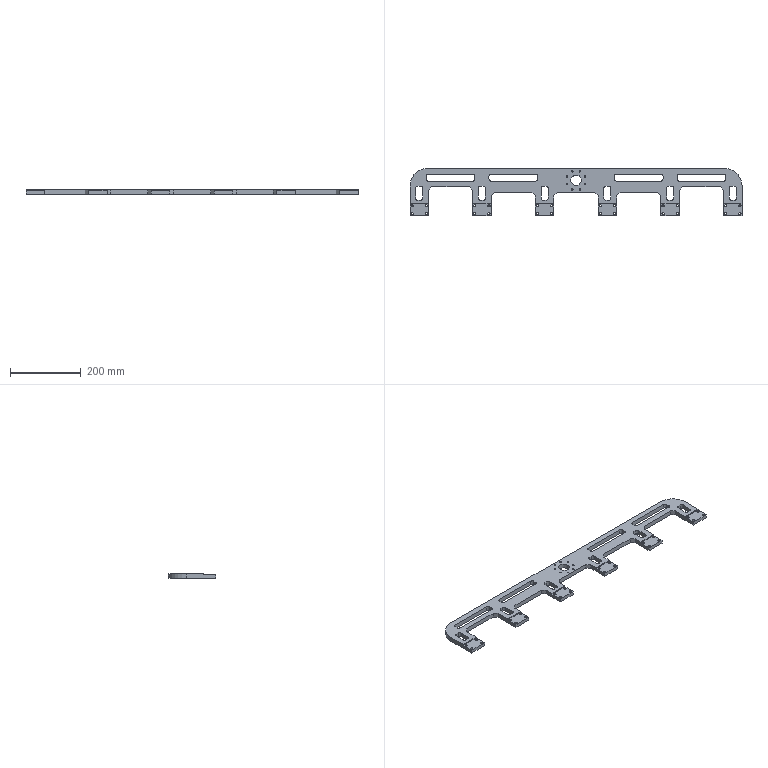NC program | NX | posted with a generic post | part box 941 x 134 x 13 mm
Lines 100 to 1108 of 8798:
(ZLEVEL_PROFILE_COPY_3 , TOOL : D10)
N180 T10 M6
N182 G54
N184 G17 G0 G90 X65.687 Y-75.6 S9500 M3
N186 G43 Z30. H10
N188 Z4.036
N190 G94 G1 Z-0.964 F1000.
N192 X63.955 Y-72.6
N194 G3 X63.089 Y-72.1 R1.
N196 G1 X62.9 F3500.
N198 G2 X57.8 Y-67. R5.1
N200 G1 Y-13.067
N202 X50.788 Y-6.055
N204 X-50.788
N206 X-57.8 Y-13.067
N208 Y-67.
N210 G2 X-62.9 Y-72.1 R5.1
N212 G1 X-114.9
N214 G2 X-120. Y-67. R5.1
N216 G1 Y-13.067
N218 X-127.012 Y-6.055
N220 X-228.588
N222 X-235.6 Y-13.067
N224 Y-67.
N226 G2 X-240.7 Y-72.1 R5.1
N228 G1 X-292.7
N230 G2 X-297.8 Y-67. R5.1
N232 G1 Y2.888
N234 X-304.812 Y9.9
N236 X-406.388
N238 X-413.4 Y2.888
N240 Y-67.
N242 G2 X-418.5 Y-72.1 R5.1
N244 G1 X-470.5
N246 G2 X-475.6 Y-67. R5.1
N248 G1 Y17.
N250 G2 X-420.5 Y72.1 R55.1
N252 G1 X63.089
N254 G3 X63.955 Y72.6 R1.
N256 G1 X65.687 Y75.6
N258 Z4.036
N260 G0 Z30.
N262 Z3.071
N264 G1 Z-1.929 F1000.
N266 X63.955 Y72.6
N268 G2 X63.089 Y72.1 R1.
N270 G1 X-420.5 F3500.
N272 G3 X-475.6 Y17. R55.1
N274 G1 Y-67.
N276 G3 X-470.5 Y-72.1 R5.1
N278 G1 X-418.5
N280 G3 X-413.4 Y-67. R5.1
N282 G1 Y2.888
N284 X-406.388 Y9.9
N286 X-304.812
N288 X-297.8 Y2.888
N290 Y-67.
N292 G3 X-292.7 Y-72.1 R5.1
N294 G1 X-240.7
N296 G3 X-235.6 Y-67. R5.1
N298 G1 Y-13.067
N300 X-228.588 Y-6.055
N302 X-127.012
N304 X-120. Y-13.067
N306 Y-67.
N308 G3 X-114.9 Y-72.1 R5.1
N310 G1 X-62.9
N312 G3 X-57.8 Y-67. R5.1
N314 G1 Y-13.067
N316 X-50.788 Y-6.055
N318 X50.788
N320 X57.8 Y-13.067
N322 Y-67.
N324 G3 X62.9 Y-72.1 R5.1
N326 G1 X63.089
N328 G2 X63.955 Y-72.6 R1.
N330 G1 X65.687 Y-75.6
N332 Z3.071
N334 G0 Z30.
N336 Z2.107
N338 G1 Z-2.893 F1000.
N340 X63.955 Y-72.6
N342 G3 X63.089 Y-72.1 R1.
N344 G1 X62.9 F3500.
N346 G2 X57.8 Y-67. R5.1
N348 G1 Y-13.067
N350 X50.788 Y-6.055
N352 X-50.788
N354 X-57.8 Y-13.067
N356 Y-67.
N358 G2 X-62.9 Y-72.1 R5.1
N360 G1 X-114.9
N362 G2 X-120. Y-67. R5.1
N364 G1 Y-13.067
N366 X-127.012 Y-6.055
N368 X-228.588
N370 X-235.6 Y-13.067
N372 Y-67.
N374 G2 X-240.7 Y-72.1 R5.1
N376 G1 X-292.7
N378 G2 X-297.8 Y-67. R5.1
N380 G1 Y2.888
N382 X-304.812 Y9.9
N384 X-406.388
N386 X-413.4 Y2.888
N388 Y-67.
N390 G2 X-418.5 Y-72.1 R5.1
N392 G1 X-470.5
N394 G2 X-475.6 Y-67. R5.1
N396 G1 Y17.
N398 G2 X-420.5 Y72.1 R55.1
N400 G1 X63.089
N402 G3 X63.955 Y72.6 R1.
N404 G1 X65.687 Y75.6
N406 Z2.107
N408 G0 Z30.
N410 Z1.143
N412 G1 Z-3.857 F1000.
N414 X63.955 Y72.6
N416 G2 X63.089 Y72.1 R1.
N418 G1 X-420.5 F3500.
N420 G3 X-475.6 Y17. R55.1
N422 G1 Y-67.
N424 G3 X-470.5 Y-72.1 R5.1
N426 G1 X-418.5
N428 G3 X-413.4 Y-67. R5.1
N430 G1 Y2.888
N432 X-406.388 Y9.9
N434 X-304.812
N436 X-297.8 Y2.888
N438 Y-67.
N440 G3 X-292.7 Y-72.1 R5.1
N442 G1 X-240.7
N444 G3 X-235.6 Y-67. R5.1
N446 G1 Y-13.067
N448 X-228.588 Y-6.055
N450 X-127.012
N452 X-120. Y-13.067
N454 Y-67.
N456 G3 X-114.9 Y-72.1 R5.1
N458 G1 X-62.9
N460 G3 X-57.8 Y-67. R5.1
N462 G1 Y-13.067
N464 X-50.788 Y-6.055
N466 X50.788
N468 X57.8 Y-13.067
N470 Y-67.
N472 G3 X62.9 Y-72.1 R5.1
N474 G1 X63.089
N476 G2 X63.955 Y-72.6 R1.
N478 G1 X65.687 Y-75.6
N480 Z1.143
N482 G0 Z30.
N484 Z0.179
N486 G1 Z-4.821 F1000.
N488 X63.955 Y-72.6
N490 G3 X63.089 Y-72.1 R1.
N492 G1 X62.9 F3500.
N494 G2 X57.8 Y-67. R5.1
N496 G1 Y-13.067
N498 X50.788 Y-6.055
N500 X-50.788
N502 X-57.8 Y-13.067
N504 Y-67.
N506 G2 X-62.9 Y-72.1 R5.1
N508 G1 X-114.9
N510 G2 X-120. Y-67. R5.1
N512 G1 Y-13.067
N514 X-127.012 Y-6.055
N516 X-228.588
N518 X-235.6 Y-13.067
N520 Y-67.
N522 G2 X-240.7 Y-72.1 R5.1
N524 G1 X-292.7
N526 G2 X-297.8 Y-67. R5.1
N528 G1 Y2.888
N530 X-304.812 Y9.9
N532 X-406.388
N534 X-413.4 Y2.888
N536 Y-67.
N538 G2 X-418.5 Y-72.1 R5.1
N540 G1 X-470.5
N542 G2 X-475.6 Y-67. R5.1
N544 G1 Y17.
N546 G2 X-420.5 Y72.1 R55.1
N548 G1 X63.089
N550 G3 X63.955 Y72.6 R1.
N552 G1 X65.687 Y75.6
N554 Z0.179
N556 G0 Z30.
N558 Z-0.786
N560 G1 Z-5.786 F1000.
N562 X63.955 Y72.6
N564 G2 X63.089 Y72.1 R1.
N566 G1 X-420.5 F3500.
N568 G3 X-475.6 Y17. R55.1
N570 G1 Y-67.
N572 G3 X-470.5 Y-72.1 R5.1
N574 G1 X-418.5
N576 G3 X-413.4 Y-67. R5.1
N578 G1 Y2.888
N580 X-406.388 Y9.9
N582 X-304.812
N584 X-297.8 Y2.888
N586 Y-67.
N588 G3 X-292.7 Y-72.1 R5.1
N590 G1 X-240.7
N592 G3 X-235.6 Y-67. R5.1
N594 G1 Y-13.067
N596 X-228.588 Y-6.055
N598 X-127.012
N600 X-120. Y-13.067
N602 Y-67.
N604 G3 X-114.9 Y-72.1 R5.1
N606 G1 X-62.9
N608 G3 X-57.8 Y-67. R5.1
N610 G1 Y-13.067
N612 X-50.788 Y-6.055
N614 X50.788
N616 X57.8 Y-13.067
N618 Y-67.
N620 G3 X62.9 Y-72.1 R5.1
N622 G1 X63.089
N624 G2 X63.955 Y-72.6 R1.
N626 G1 X65.687 Y-75.6
N628 Z-0.786
N630 G0 Z30.
N632 Z-1.75
N634 G1 Z-6.75 F1000.
N636 X63.955 Y-72.6
N638 G3 X63.089 Y-72.1 R1.
N640 G1 X62.9 F3500.
N642 G2 X57.8 Y-67. R5.1
N644 G1 Y-13.067
N646 X50.788 Y-6.055
N648 X-50.788
N650 X-57.8 Y-13.067
N652 Y-67.
N654 G2 X-62.9 Y-72.1 R5.1
N656 G1 X-114.9
N658 G2 X-120. Y-67. R5.1
N660 G1 Y-13.067
N662 X-127.012 Y-6.055
N664 X-228.588
N666 X-235.6 Y-13.067
N668 Y-67.
N670 G2 X-240.7 Y-72.1 R5.1
N672 G1 X-292.7
N674 G2 X-297.8 Y-67. R5.1
N676 G1 Y2.888
N678 X-304.812 Y9.9
N680 X-406.388
N682 X-413.4 Y2.888
N684 Y-67.
N686 G2 X-418.5 Y-72.1 R5.1
N688 G1 X-470.5
N690 G2 X-475.6 Y-67. R5.1
N692 G1 Y17.
N694 G2 X-420.5 Y72.1 R55.1
N696 G1 X63.089
N698 G3 X63.955 Y72.6 R1.
N700 G1 X65.687 Y75.6
N702 Z-1.75
N704 G0 Z30.
N706 Z-2.714
N708 G1 Z-7.714 F1000.
N710 X63.955 Y72.6
N712 G2 X63.089 Y72.1 R1.
N714 G1 X-420.5 F3500.
N716 G3 X-475.6 Y17. R55.1
N718 G1 Y-67.
N720 G3 X-470.5 Y-72.1 R5.1
N722 G1 X-418.5
N724 G3 X-413.4 Y-67. R5.1
N726 G1 Y2.888
N728 X-406.388 Y9.9
N730 X-304.812
N732 X-297.8 Y2.888
N734 Y-67.
N736 G3 X-292.7 Y-72.1 R5.1
N738 G1 X-240.7
N740 G3 X-235.6 Y-67. R5.1
N742 G1 Y-13.067
N744 X-228.588 Y-6.055
N746 X-127.012
N748 X-120. Y-13.067
N750 Y-67.
N752 G3 X-114.9 Y-72.1 R5.1
N754 G1 X-62.9
N756 G3 X-57.8 Y-67. R5.1
N758 G1 Y-13.067
N760 X-50.788 Y-6.055
N762 X50.788
N764 X57.8 Y-13.067
N766 Y-67.
N768 G3 X62.9 Y-72.1 R5.1
N770 G1 X63.089
N772 G2 X63.955 Y-72.6 R1.
N774 G1 X65.687 Y-75.6
N776 Z-2.714
N778 G0 Z30.
N780 Z-3.679
N782 G1 Z-8.679 F1000.
N784 X63.955 Y-72.6
N786 G3 X63.089 Y-72.1 R1.
N788 G1 X62.9 F3500.
N790 G2 X57.8 Y-67. R5.1
N792 G1 Y-13.067
N794 X50.788 Y-6.055
N796 X-50.788
N798 X-57.8 Y-13.067
N800 Y-67.
N802 G2 X-62.9 Y-72.1 R5.1
N804 G1 X-114.9
N806 G2 X-120. Y-67. R5.1
N808 G1 Y-13.067
N810 X-127.012 Y-6.055
N812 X-228.588
N814 X-235.6 Y-13.067
N816 Y-67.
N818 G2 X-240.7 Y-72.1 R5.1
N820 G1 X-292.7
N822 G2 X-297.8 Y-67. R5.1
N824 G1 Y2.888
N826 X-304.812 Y9.9
N828 X-406.388
N830 X-413.4 Y2.888
N832 Y-67.
N834 G2 X-418.5 Y-72.1 R5.1
N836 G1 X-470.5
N838 G2 X-475.6 Y-67. R5.1
N840 G1 Y17.
N842 G2 X-420.5 Y72.1 R55.1
N844 G1 X63.089
N846 G3 X63.955 Y72.6 R1.
N848 G1 X65.687 Y75.6
N850 Z-3.679
N852 G0 Z30.
N854 Z-4.643
N856 G1 Z-9.643 F1000.
N858 X63.955 Y72.6
N860 G2 X63.089 Y72.1 R1.
N862 G1 X-420.5 F3500.
N864 G3 X-475.6 Y17. R55.1
N866 G1 Y-67.
N868 G3 X-470.5 Y-72.1 R5.1
N870 G1 X-418.5
N872 G3 X-413.4 Y-67. R5.1
N874 G1 Y2.888
N876 X-406.388 Y9.9
N878 X-304.812
N880 X-297.8 Y2.888
N882 Y-67.
N884 G3 X-292.7 Y-72.1 R5.1
N886 G1 X-240.7
N888 G3 X-235.6 Y-67. R5.1
N890 G1 Y-13.067
N892 X-228.588 Y-6.055
N894 X-127.012
N896 X-120. Y-13.067
N898 Y-67.
N900 G3 X-114.9 Y-72.1 R5.1
N902 G1 X-62.9
N904 G3 X-57.8 Y-67. R5.1
N906 G1 Y-13.067
N908 X-50.788 Y-6.055
N910 X50.788
N912 X57.8 Y-13.067
N914 Y-67.
N916 G3 X62.9 Y-72.1 R5.1
N918 G1 X63.089
N920 G2 X63.955 Y-72.6 R1.
N922 G1 X65.687 Y-75.6
N924 Z-4.643
N926 G0 Z30.
N928 Z-5.607
N930 G1 Z-10.607 F1000.
N932 X63.955 Y-72.6
N934 G3 X63.089 Y-72.1 R1.
N936 G1 X62.9 F3500.
N938 G2 X57.8 Y-67. R5.1
N940 G1 Y-13.067
N942 X50.788 Y-6.055
N944 X-50.788
N946 X-57.8 Y-13.067
N948 Y-67.
N950 G2 X-62.9 Y-72.1 R5.1
N952 G1 X-114.9
N954 G2 X-120. Y-67. R5.1
N956 G1 Y-13.067
N958 X-127.012 Y-6.055
N960 X-228.588
N962 X-235.6 Y-13.067
N964 Y-67.
N966 G2 X-240.7 Y-72.1 R5.1
N968 G1 X-292.7
N970 G2 X-297.8 Y-67. R5.1
N972 G1 Y2.888
N974 X-304.812 Y9.9
N976 X-406.388
N978 X-413.4 Y2.888
N980 Y-67.
N982 G2 X-418.5 Y-72.1 R5.1
N984 G1 X-470.5
N986 G2 X-475.6 Y-67. R5.1
N988 G1 Y17.
N990 G2 X-420.5 Y72.1 R55.1
N992 G1 X63.089
N994 G3 X63.955 Y72.6 R1.
N996 G1 X65.687 Y75.6
N998 Z-5.607
N1000 G0 Z30.
N1002 Z-6.571
N1004 G1 Z-11.571 F1000.
N1006 X63.955 Y72.6
N1008 G2 X63.089 Y72.1 R1.
N1010 G1 X-420.5 F3500.
N1012 G3 X-475.6 Y17. R55.1
N1014 G1 Y-67.
N1016 G3 X-470.5 Y-72.1 R5.1
N1018 G1 X-418.5
N1020 G3 X-413.4 Y-67. R5.1
N1022 G1 Y2.888
N1024 X-406.388 Y9.9
N1026 X-304.812
N1028 X-297.8 Y2.888
N1030 Y-67.
N1032 G3 X-292.7 Y-72.1 R5.1
N1034 G1 X-240.7
N1036 G3 X-235.6 Y-67. R5.1
N1038 G1 Y-13.067
N1040 X-228.588 Y-6.055
N1042 X-127.012
N1044 X-120. Y-13.067
N1046 Y-67.
N1048 G3 X-114.9 Y-72.1 R5.1
N1050 G1 X-62.9
N1052 G3 X-57.8 Y-67. R5.1
N1054 G1 Y-13.067
N1056 X-50.788 Y-6.055
N1058 X50.788
N1060 X57.8 Y-13.067
N1062 Y-67.
N1064 G3 X62.9 Y-72.1 R5.1
N1066 G1 X63.089
N1068 G2 X63.955 Y-72.6 R1.
N1070 G1 X65.687 Y-75.6
N1072 Z-6.571
N1074 G0 Z30.
N1076 Z-7.536
N1078 G1 Z-12.536 F1000.
N1080 X63.955 Y-72.6
N1082 G3 X63.089 Y-72.1 R1.
N1084 G1 X62.9 F3500.
N1086 G2 X57.8 Y-67. R5.1
N1088 G1 Y-13.067
N1090 X50.788 Y-6.055
N1092 X-50.788
N1094 X-57.8 Y-13.067
N1096 Y-67.
N1098 G2 X-62.9 Y-72.1 R5.1
N1100 G1 X-114.9
N1102 G2 X-120. Y-67. R5.1
N1104 G1 Y-13.067
N1106 X-127.012 Y-6.055
N1108 X-228.588
N1110 X-235.6 Y-13.067
N1112 Y-67.
N1114 G2 X-240.7 Y-72.1 R5.1
N1116 G1 X-292.7
N1118 G2 X-297.8 Y-67. R5.1
N1120 G1 Y2.888
N1122 X-304.812 Y9.9
N1124 X-406.388
N1126 X-413.4 Y2.888
N1128 Y-67.
N1130 G2 X-418.5 Y-72.1 R5.1
N1132 G1 X-470.5
N1134 G2 X-475.6 Y-67. R5.1
N1136 G1 Y17.
N1138 G2 X-420.5 Y72.1 R55.1
N1140 G1 X63.089
N1142 G3 X63.955 Y72.6 R1.
N1144 G1 X65.687 Y75.6
N1146 Z-7.536
N1148 G0 Z30.
N1150 Z-8.5
N1152 G1 Z-13.5 F1000.
N1154 X63.955 Y72.6
N1156 G2 X63.089 Y72.1 R1.
N1158 G1 X-420.5 F3500.
N1160 G3 X-475.6 Y17. R55.1
N1162 G1 Y-67.
N1164 G3 X-470.5 Y-72.1 R5.1
N1166 G1 X-418.5
N1168 G3 X-413.4 Y-67. R5.1
N1170 G1 Y2.888
N1172 X-406.388 Y9.9
N1174 X-304.812
N1176 X-297.8 Y2.888
N1178 Y-67.
N1180 G3 X-292.7 Y-72.1 R5.1
N1182 G1 X-240.7
N1184 G3 X-235.6 Y-67. R5.1
N1186 G1 Y-13.067
N1188 X-228.588 Y-6.055
N1190 X-127.012
N1192 X-120. Y-13.067
N1194 Y-67.
N1196 G3 X-114.9 Y-72.1 R5.1
N1198 G1 X-62.9
N1200 G3 X-57.8 Y-67. R5.1
N1202 G1 Y-13.067
N1204 X-50.788 Y-6.055
N1206 X50.788
N1208 X57.8 Y-13.067
N1210 Y-67.
N1212 G3 X62.9 Y-72.1 R5.1
N1214 G1 X63.089
N1216 G2 X63.955 Y-72.6 R1.
N1218 G1 X65.687 Y-75.6
N1220 Z-8.5
N1222 G0 Z30.
(ZLEVEL_PROFILE_COPY_3_COPY , TOOL : D10)
N1224 Y-75.5
N1226 Z-8.5
N1228 G1 Z-13.5 F1000.
N1230 X63.955 Y-72.5
N1232 G3 X63.089 Y-72. R1.
N1234 G1 X62.9 F1200.
N1236 G2 X57.9 Y-67. R5.
N1238 G1 Y-13.026
N1240 X50.829 Y-5.955
N1242 X-50.829
N1244 X-57.9 Y-13.026
N1246 Y-67.
N1248 G2 X-62.9 Y-72. R5.
N1250 G1 X-114.9
N1252 G2 X-119.9 Y-67. R5.
N1254 G1 Y-13.026
N1256 X-126.971 Y-5.955
N1258 X-228.629
N1260 X-235.7 Y-13.026
N1262 Y-67.
N1264 G2 X-240.7 Y-72. R5.
N1266 G1 X-292.7
N1268 G2 X-297.7 Y-67. R5.
N1270 G1 Y2.929
N1272 X-304.771 Y10.
N1274 X-406.429
N1276 X-413.5 Y2.929
N1278 Y-67.
N1280 G2 X-418.5 Y-72. R5.
N1282 G1 X-470.5
N1284 G2 X-475.5 Y-67. R5.
N1286 G1 Y17.
N1288 G2 X-420.5 Y72. R55.
N1290 G1 X63.089
N1292 G3 X63.955 Y72.5 R1.
N1294 G1 X65.687 Y75.5
N1296 Z-8.5
N1298 G0 Z30.
(ZLEVEL_PROFILE_COPY_2_COPY_COPY , TOOL : D10)
N1300 X0.245 Y28.007
N1302 Z1.5
N1304 G1 X0.513 Z1.486 F1000.
N1306 X1.326 Y28.142 Z1.443
N1308 X2.106 Y28.409 Z1.4
N1310 X2.832 Y28.8 Z1.356
N1312 X3.483 Y29.305 Z1.313
N1314 X4.044 Y29.91 Z1.27
N1316 X4.402 Y30.432 Z1.237
N1318 X4.776 Y31.2 Z1.192
N1320 X5.014 Y32.022 Z1.147
N1322 X5.108 Y32.871 Z1.102
N1324 X5.057 Y33.725 Z1.058
N1326 X4.862 Y34.557 Z1.013
N1328 X4.528 Y35.344 Z0.968
N1330 X4.065 Y36.063 Z0.923
N1332 X3.486 Y36.693 Z0.878
N1334 X2.809 Y37.215 Z0.834
N1336 X2.053 Y37.614 Z0.789
N1338 X1.456 Y37.823 Z0.756
N1340 X0.941 Y37.939 Z0.728
N1342 X0.416 Y38. Z0.7
N1344 X-0.216 Z0.667
N1346 X-0.532 Y37.97 Z0.65
N1348 X-1.154 Y37.851 Z0.617
N1350 X-1.951 Y37.571 Z0.573
N1352 X-2.689 Y37.162 Z0.529
N1354 X-3.349 Y36.634 Z0.484
N1356 X-3.91 Y36.003 Z0.44
N1358 X-4.358 Y35.287 Z0.396
N1360 X-4.678 Y34.506 Z0.352
N1362 X-4.863 Y33.682 Z0.307
N1364 X-4.907 Y32.838 Z0.263
N1366 X-4.809 Y31.999 Z0.219
N1368 X-4.571 Y31.189 Z0.175
N1370 X-4.201 Y30.43 Z0.13
N1372 X-3.842 Y29.908 Z0.097
N1374 X-3.282 Y29.304 Z0.054
N1376 X-2.63 Y28.799 Z0.011
N1378 X-1.904 Y28.408 Z-0.032
N1380 X-1.124 Y28.142 Z-0.076
N1382 X-0.311 Y28.007 Z-0.119
N1384 X0.513 Z-0.162
N1386 X1.326 Y28.142 Z-0.205
N1388 X2.106 Y28.409 Z-0.248
N1390 X2.832 Y28.8 Z-0.292
N1392 X3.483 Y29.305 Z-0.335
N1394 X4.044 Y29.91 Z-0.378
N1396 X4.402 Y30.432 Z-0.411
N1398 X4.776 Y31.2 Z-0.456
N1400 X5.014 Y32.022 Z-0.501
N1402 X5.108 Y32.871 Z-0.546
N1404 X5.057 Y33.725 Z-0.59
N1406 X4.862 Y34.557 Z-0.635
N1408 X4.528 Y35.344 Z-0.68
N1410 X4.065 Y36.063 Z-0.725
N1412 X3.486 Y36.693 Z-0.77
N1414 X2.809 Y37.215 Z-0.814
N1416 X2.053 Y37.614 Z-0.859
N1418 X1.456 Y37.823 Z-0.892
N1420 X0.941 Y37.939 Z-0.92
N1422 X0.416 Y38. Z-0.948
N1424 X0.1 Z-0.964
N1426 G3 X-4.9 Y33. R5. F2000.
N1428 X0.1 Y38. R-5.
N1430 G1 X-0.209 Y37.984 Z-0.977
N1432 X-0.518 Y37.956 Z-0.99
N1434 X-0.823 Y37.907 Z-1.002
N1436 X-1.125 Y37.839 Z-1.015
N1438 X-1.423 Y37.754 Z-1.028
N1440 X-1.715 Y37.65 Z-1.04
N1442 X-2. Y37.529 Z-1.053
N1444 X-2.276 Y37.391 Z-1.066
N1446 X-2.411 Y37.314 Z-1.072
N1448 X-2.545 Y37.237 Z-1.078
N1450 X-2.673 Y37.151 Z-1.085
N1452 X-2.801 Y37.064 Z-1.091
N1454 X-3.047 Y36.875 Z-1.104
N1456 X-3.281 Y36.673 Z-1.117
N1458 X-3.502 Y36.456 Z-1.129
N1460 X-3.709 Y36.226 Z-1.142
N1462 X-3.903 Y35.985 Z-1.155
N1464 X-4.081 Y35.732 Z-1.167
N1466 X-4.241 Y35.467 Z-1.18
N1468 X-4.385 Y35.192 Z-1.193
N1470 X-4.512 Y34.91 Z-1.205
N1472 X-4.621 Y34.621 Z-1.218
N1474 X-4.713 Y34.325 Z-1.231
N1476 X-4.787 Y34.025 Z-1.243
N1478 X-4.815 Y33.872 Z-1.25
N1480 X-4.842 Y33.72 Z-1.256
N1482 X-4.86 Y33.566 Z-1.262
N1484 X-4.876 Y33.412 Z-1.269
N1486 X-4.891 Y33.103 Z-1.281
N1488 X-4.888 Y32.794 Z-1.294
N1490 X-4.887 Y32.638 Z-1.301
N1492 X-4.873 Y32.484 Z-1.307
N1494 X-4.855 Y32.33 Z-1.313
N1496 X-4.832 Y32.177 Z-1.32
N1498 X-4.771 Y31.873 Z-1.332
N1500 X-4.692 Y31.573 Z-1.345
N1502 X-4.595 Y31.279 Z-1.358
N1504 X-4.479 Y30.992 Z-1.37
N1506 X-4.346 Y30.712 Z-1.383
N1508 X-4.195 Y30.441 Z-1.396
N1510 X-4.028 Y30.179 Z-1.408
N1512 X-3.846 Y29.929 Z-1.421
N1514 X-3.648 Y29.69 Z-1.434
N1516 X-3.436 Y29.464 Z-1.446
N1518 X-3.205 Y29.258 Z-1.459
N1520 X-2.966 Y29.061 Z-1.472
N1522 X-2.716 Y28.878 Z-1.484
N1524 X-2.455 Y28.712 Z-1.497
N1526 X-2.185 Y28.561 Z-1.51
N1528 X-1.906 Y28.426 Z-1.523
N1530 X-1.619 Y28.312 Z-1.535
N1532 X-1.324 Y28.216 Z-1.548
N1534 X-1.025 Y28.137 Z-1.561
N1536 X-0.722 Y28.076 Z-1.573
N1538 X-0.415 Y28.034 Z-1.586
N1540 X-0.106 Y28.009 Z-1.599
N1542 X0.203 Y28.007 Z-1.611
N1544 X0.512 Y28.024 Z-1.624
N1546 X0.82 Y28.06 Z-1.637
N1548 X1.124 Y28.114 Z-1.649
N1550 X1.425 Y28.187 Z-1.662
N1552 X1.721 Y28.279 Z-1.675
N1554 X2.011 Y28.387 Z-1.688
N1556 X2.294 Y28.513 Z-1.7
N1558 X2.567 Y28.659 Z-1.713
N1560 X2.83 Y28.821 Z-1.726
N1562 X3.084 Y28.998 Z-1.738
N1564 X3.326 Y29.191 Z-1.751
N1566 X3.556 Y29.398 Z-1.764
N1568 X3.774 Y29.618 Z-1.776
N1570 X3.876 Y29.735 Z-1.783
N1572 X3.977 Y29.852 Z-1.789
N1574 X4.071 Y29.975 Z-1.795
N1576 X4.164 Y30.099 Z-1.802
N1578 X4.335 Y30.356 Z-1.814
N1580 X4.49 Y30.624 Z-1.827
N1582 X4.629 Y30.901 Z-1.84
N1584 X4.75 Y31.185 Z-1.852
N1586 X4.855 Y31.477 Z-1.865
N1588 X4.942 Y31.774 Z-1.878
N1590 X4.974 Y31.925 Z-1.884
N1592 X5.008 Y32.076 Z-1.891
N1594 X5.031 Y32.229 Z-1.897
N1596 X5.054 Y32.383 Z-1.903
N1598 X5.082 Y32.691 Z-1.916
N1600 X5.1 Y33. Z-1.929
N1602 G3 X0.1 Y38. R5.
N1604 G1 X-0.209 Y37.984 Z-1.941
N1606 X-0.518 Y37.956 Z-1.954
N1608 X-0.823 Y37.907 Z-1.967
N1610 X-1.125 Y37.839 Z-1.979
N1612 X-1.423 Y37.754 Z-1.992
N1614 X-1.715 Y37.65 Z-2.005
N1616 X-2. Y37.529 Z-2.017
N1618 X-2.276 Y37.391 Z-2.03
N1620 X-2.411 Y37.314 Z-2.036
N1622 X-2.545 Y37.237 Z-2.043
N1624 X-2.673 Y37.151 Z-2.049
N1626 X-2.801 Y37.064 Z-2.055
N1628 X-3.047 Y36.875 Z-2.068
N1630 X-3.281 Y36.673 Z-2.081
N1632 X-3.502 Y36.456 Z-2.094
N1634 X-3.709 Y36.226 Z-2.106
N1636 X-3.903 Y35.985 Z-2.119
N1638 X-4.081 Y35.732 Z-2.132
N1640 X-4.241 Y35.467 Z-2.144
N1642 X-4.385 Y35.192 Z-2.157
N1644 X-4.512 Y34.91 Z-2.17
N1646 X-4.621 Y34.621 Z-2.182
N1648 X-4.713 Y34.325 Z-2.195
N1650 X-4.787 Y34.025 Z-2.208
N1652 X-4.815 Y33.872 Z-2.214
N1654 X-4.842 Y33.72 Z-2.22
N1656 X-4.86 Y33.566 Z-2.227
N1658 X-4.876 Y33.412 Z-2.233
N1660 X-4.891 Y33.103 Z-2.246
N1662 X-4.888 Y32.794 Z-2.258
N1664 X-4.887 Y32.638 Z-2.265
N1666 X-4.873 Y32.484 Z-2.271
N1668 X-4.855 Y32.33 Z-2.277
N1670 X-4.832 Y32.177 Z-2.284
N1672 X-4.771 Y31.873 Z-2.297
N1674 X-4.692 Y31.573 Z-2.309
N1676 X-4.595 Y31.279 Z-2.322
N1678 X-4.479 Y30.992 Z-2.335
N1680 X-4.346 Y30.712 Z-2.347
N1682 X-4.195 Y30.441 Z-2.36
N1684 X-4.028 Y30.179 Z-2.373
N1686 X-3.846 Y29.929 Z-2.385
N1688 X-3.648 Y29.69 Z-2.398
N1690 X-3.436 Y29.464 Z-2.411
N1692 X-3.205 Y29.258 Z-2.423
N1694 X-2.966 Y29.061 Z-2.436
N1696 X-2.716 Y28.878 Z-2.449
N1698 X-2.455 Y28.712 Z-2.461
N1700 X-2.185 Y28.561 Z-2.474
N1702 X-1.906 Y28.426 Z-2.487
N1704 X-1.619 Y28.312 Z-2.5
N1706 X-1.324 Y28.216 Z-2.512
N1708 X-1.025 Y28.137 Z-2.525
N1710 X-0.722 Y28.076 Z-2.538
N1712 X-0.415 Y28.034 Z-2.55
N1714 X-0.106 Y28.009 Z-2.563
N1716 X0.203 Y28.007 Z-2.576
N1718 X0.512 Y28.024 Z-2.588
N1720 X0.82 Y28.06 Z-2.601
N1722 X1.124 Y28.114 Z-2.614
N1724 X1.425 Y28.187 Z-2.626
N1726 X1.721 Y28.279 Z-2.639
N1728 X2.011 Y28.387 Z-2.652
N1730 X2.294 Y28.513 Z-2.664
N1732 X2.567 Y28.659 Z-2.677
N1734 X2.83 Y28.821 Z-2.69
N1736 X3.084 Y28.998 Z-2.703
N1738 X3.326 Y29.191 Z-2.715
N1740 X3.556 Y29.398 Z-2.728
N1742 X3.774 Y29.618 Z-2.741
N1744 X3.876 Y29.735 Z-2.747
N1746 X3.977 Y29.852 Z-2.753
N1748 X4.071 Y29.975 Z-2.76
N1750 X4.164 Y30.099 Z-2.766
N1752 X4.335 Y30.356 Z-2.779
N1754 X4.49 Y30.624 Z-2.791
N1756 X4.629 Y30.901 Z-2.804
N1758 X4.75 Y31.185 Z-2.817
N1760 X4.855 Y31.477 Z-2.829
N1762 X4.942 Y31.774 Z-2.842
N1764 X4.974 Y31.925 Z-2.848
N1766 X5.008 Y32.076 Z-2.855
N1768 X5.031 Y32.229 Z-2.861
N1770 X5.054 Y32.383 Z-2.867
N1772 X5.082 Y32.691 Z-2.88
N1774 X5.1 Y33. Z-2.893
N1776 G3 X0.1 Y38. R5.
N1778 G1 X-0.209 Y37.984 Z-2.906
N1780 X-0.518 Y37.956 Z-2.918
N1782 X-0.823 Y37.907 Z-2.931
N1784 X-1.125 Y37.839 Z-2.944
N1786 X-1.423 Y37.754 Z-2.956
N1788 X-1.715 Y37.65 Z-2.969
N1790 X-1.999 Y37.529 Z-2.982
N1792 X-2.276 Y37.391 Z-2.994
N1794 X-2.411 Y37.314 Z-3.001
N1796 X-2.545 Y37.237 Z-3.007
N1798 X-2.673 Y37.151 Z-3.013
N1800 X-2.801 Y37.064 Z-3.02
N1802 X-3.047 Y36.875 Z-3.032
N1804 X-3.281 Y36.673 Z-3.045
N1806 X-3.502 Y36.456 Z-3.058
N1808 X-3.709 Y36.226 Z-3.07
N1810 X-3.903 Y35.985 Z-3.083
N1812 X-4.081 Y35.732 Z-3.096
N1814 X-4.241 Y35.467 Z-3.109
N1816 X-4.385 Y35.192 Z-3.121
N1818 X-4.512 Y34.91 Z-3.134
N1820 X-4.621 Y34.621 Z-3.147
N1822 X-4.713 Y34.325 Z-3.159
N1824 X-4.787 Y34.025 Z-3.172
N1826 X-4.815 Y33.872 Z-3.178
N1828 X-4.842 Y33.72 Z-3.185
N1830 X-4.86 Y33.566 Z-3.191
N1832 X-4.876 Y33.412 Z-3.197
N1834 X-4.891 Y33.103 Z-3.21
N1836 X-4.888 Y32.794 Z-3.223
N1838 X-4.887 Y32.638 Z-3.229
N1840 X-4.873 Y32.484 Z-3.235
N1842 X-4.855 Y32.33 Z-3.242
N1844 X-4.832 Y32.177 Z-3.248
N1846 X-4.771 Y31.873 Z-3.261
N1848 X-4.692 Y31.573 Z-3.273
N1850 X-4.595 Y31.279 Z-3.286
N1852 X-4.479 Y30.992 Z-3.299
N1854 X-4.346 Y30.712 Z-3.312
N1856 X-4.195 Y30.441 Z-3.324
N1858 X-4.028 Y30.179 Z-3.337
N1860 X-3.846 Y29.929 Z-3.35
N1862 X-3.648 Y29.69 Z-3.362
N1864 X-3.436 Y29.464 Z-3.375
N1866 X-3.205 Y29.258 Z-3.388
N1868 X-2.966 Y29.061 Z-3.4
N1870 X-2.716 Y28.878 Z-3.413
N1872 X-2.455 Y28.712 Z-3.426
N1874 X-2.185 Y28.561 Z-3.438
N1876 X-1.906 Y28.426 Z-3.451
N1878 X-1.619 Y28.312 Z-3.464
N1880 X-1.324 Y28.216 Z-3.477
N1882 X-1.025 Y28.137 Z-3.489
N1884 X-0.722 Y28.076 Z-3.502
N1886 X-0.415 Y28.034 Z-3.515
N1888 X-0.106 Y28.009 Z-3.527
N1890 X0.203 Y28.007 Z-3.54
N1892 X0.512 Y28.024 Z-3.553
N1894 X0.82 Y28.06 Z-3.565
N1896 X1.124 Y28.114 Z-3.578
N1898 X1.425 Y28.187 Z-3.591
N1900 X1.721 Y28.279 Z-3.603
N1902 X2.011 Y28.387 Z-3.616
N1904 X2.294 Y28.513 Z-3.629
N1906 X2.567 Y28.659 Z-3.641
N1908 X2.83 Y28.821 Z-3.654
N1910 X3.084 Y28.998 Z-3.667
N1912 X3.326 Y29.191 Z-3.68
N1914 X3.556 Y29.398 Z-3.692
N1916 X3.774 Y29.618 Z-3.705
N1918 X3.876 Y29.735 Z-3.711
N1920 X3.977 Y29.852 Z-3.718
N1922 X4.071 Y29.975 Z-3.724
N1924 X4.164 Y30.099 Z-3.73
N1926 X4.335 Y30.356 Z-3.743
N1928 X4.49 Y30.624 Z-3.756
N1930 X4.629 Y30.901 Z-3.768
N1932 X4.75 Y31.185 Z-3.781
N1934 X4.855 Y31.477 Z-3.794
N1936 X4.942 Y31.774 Z-3.806
N1938 X4.974 Y31.925 Z-3.813
N1940 X5.008 Y32.076 Z-3.819
N1942 X5.031 Y32.229 Z-3.825
N1944 X5.054 Y32.383 Z-3.832
N1946 X5.082 Y32.691 Z-3.844
N1948 X5.1 Y33. Z-3.857
N1950 G3 X0.1 Y38. R5.
N1952 G1 X-0.209 Y37.984 Z-3.87
N1954 X-0.518 Y37.956 Z-3.883
N1956 X-0.823 Y37.907 Z-3.895
N1958 X-1.125 Y37.839 Z-3.908
N1960 X-1.423 Y37.754 Z-3.921
N1962 X-1.715 Y37.65 Z-3.933
N1964 X-1.999 Y37.529 Z-3.946
N1966 X-2.276 Y37.391 Z-3.959
N1968 X-2.411 Y37.314 Z-3.965
N1970 X-2.545 Y37.237 Z-3.971
N1972 X-2.673 Y37.151 Z-3.978
N1974 X-2.801 Y37.064 Z-3.984
N1976 X-3.047 Y36.875 Z-3.997
N1978 X-3.281 Y36.673 Z-4.009
N1980 X-3.502 Y36.456 Z-4.022
N1982 X-3.709 Y36.226 Z-4.035
N1984 X-3.903 Y35.985 Z-4.047
N1986 X-4.081 Y35.732 Z-4.06
N1988 X-4.241 Y35.467 Z-4.073
N1990 X-4.385 Y35.192 Z-4.086
N1992 X-4.512 Y34.91 Z-4.098
N1994 X-4.621 Y34.621 Z-4.111
N1996 X-4.713 Y34.325 Z-4.124
N1998 X-4.787 Y34.025 Z-4.136
N2000 X-4.815 Y33.872 Z-4.143
N2002 X-4.842 Y33.72 Z-4.149
N2004 X-4.86 Y33.566 Z-4.155
N2006 X-4.876 Y33.412 Z-4.162
N2008 X-4.891 Y33.103 Z-4.174
N2010 X-4.888 Y32.794 Z-4.187
N2012 X-4.887 Y32.638 Z-4.193
N2014 X-4.873 Y32.484 Z-4.2
N2016 X-4.855 Y32.33 Z-4.206
N2018 X-4.832 Y32.177 Z-4.212
N2020 X-4.771 Y31.873 Z-4.225
N2022 X-4.692 Y31.573 Z-4.238
N2024 X-4.595 Y31.279 Z-4.25
N2026 X-4.479 Y30.992 Z-4.263
N2028 X-4.346 Y30.712 Z-4.276
N2030 X-4.195 Y30.441 Z-4.289
N2032 X-4.028 Y30.179 Z-4.301
N2034 X-3.846 Y29.929 Z-4.314
N2036 X-3.648 Y29.69 Z-4.327
N2038 X-3.436 Y29.464 Z-4.339
N2040 X-3.205 Y29.258 Z-4.352
N2042 X-2.966 Y29.061 Z-4.365
N2044 X-2.716 Y28.878 Z-4.377
N2046 X-2.455 Y28.712 Z-4.39
N2048 X-2.185 Y28.561 Z-4.403
N2050 X-1.906 Y28.426 Z-4.415
N2052 X-1.619 Y28.312 Z-4.428
N2054 X-1.324 Y28.216 Z-4.441
N2056 X-1.025 Y28.137 Z-4.453
N2058 X-0.722 Y28.076 Z-4.466
N2060 X-0.415 Y28.034 Z-4.479
N2062 X-0.106 Y28.009 Z-4.492
N2064 X0.203 Y28.007 Z-4.504
N2066 X0.512 Y28.024 Z-4.517
N2068 X0.82 Y28.06 Z-4.53
N2070 X1.124 Y28.114 Z-4.542
N2072 X1.425 Y28.187 Z-4.555
N2074 X1.721 Y28.279 Z-4.568
N2076 X2.011 Y28.387 Z-4.58
N2078 X2.294 Y28.513 Z-4.593
N2080 X2.567 Y28.659 Z-4.606
N2082 X2.83 Y28.821 Z-4.618
N2084 X3.084 Y28.998 Z-4.631
N2086 X3.326 Y29.191 Z-4.644
N2088 X3.556 Y29.398 Z-4.656
N2090 X3.774 Y29.618 Z-4.669
N2092 X3.876 Y29.735 Z-4.676
N2094 X3.977 Y29.852 Z-4.682
N2096 X4.071 Y29.975 Z-4.688
N2098 X4.164 Y30.099 Z-4.695
N2100 X4.335 Y30.356 Z-4.707
N2102 X4.49 Y30.624 Z-4.72
N2104 X4.629 Y30.901 Z-4.733
N2106 X4.75 Y31.185 Z-4.745
N2108 X4.855 Y31.477 Z-4.758
N2110 X4.942 Y31.774 Z-4.771
N2112 X4.974 Y31.925 Z-4.777
N2114 X5.008 Y32.076 Z-4.783
N2116 X5.031 Y32.229 Z-4.79
N2118 X5.054 Y32.383 Z-4.796
N2120 X5.082 Y32.691 Z-4.809
N2122 X5.1 Y33. Z-4.821
N2124 G3 X0.1 Y38. R5.
N2126 G1 X-0.209 Y37.984 Z-4.834
N2128 X-0.518 Y37.956 Z-4.847
N2130 X-0.823 Y37.907 Z-4.859
N2132 X-1.125 Y37.839 Z-4.872
N2134 X-1.423 Y37.754 Z-4.885
N2136 X-1.715 Y37.65 Z-4.898
N2138 X-1.999 Y37.529 Z-4.91
N2140 X-2.276 Y37.391 Z-4.923
N2142 X-2.411 Y37.314 Z-4.929
N2144 X-2.545 Y37.237 Z-4.936
N2146 X-2.673 Y37.151 Z-4.942
N2148 X-2.801 Y37.064 Z-4.948
N2150 X-3.047 Y36.875 Z-4.961
N2152 X-3.281 Y36.673 Z-4.974
N2154 X-3.502 Y36.456 Z-4.986
N2156 X-3.709 Y36.226 Z-4.999
N2158 X-3.903 Y35.985 Z-5.012
N2160 X-4.081 Y35.732 Z-5.024
N2162 X-4.241 Y35.467 Z-5.037
N2164 X-4.385 Y35.192 Z-5.05
N2166 X-4.512 Y34.91 Z-5.063
N2168 X-4.621 Y34.621 Z-5.075
N2170 X-4.713 Y34.325 Z-5.088
N2172 X-4.787 Y34.025 Z-5.101
N2174 X-4.815 Y33.872 Z-5.107
N2176 X-4.842 Y33.72 Z-5.113
N2178 X-4.86 Y33.566 Z-5.12